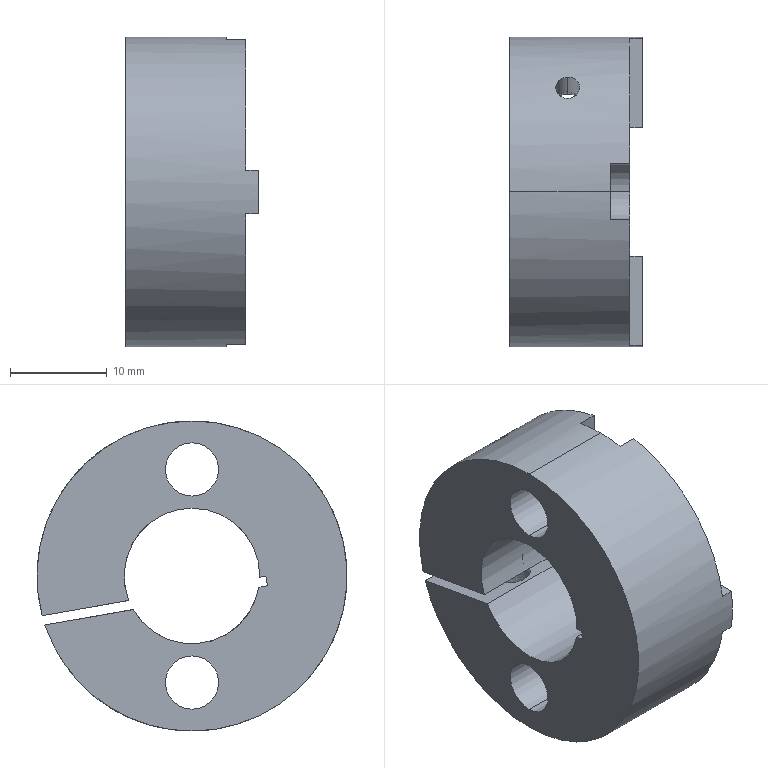Part | SolidWorks | features BaseBody 1 | 1 solid | 52 faces | box 13.7 x 32 x 32 mm | volume 6989 mm3 | cylinder 25 | plane 23 | cone 4 | commonest cylinder face diameters 2.459 x6 5.5 x6 3.9 x4 5.86 x3 14 x3 32 x3